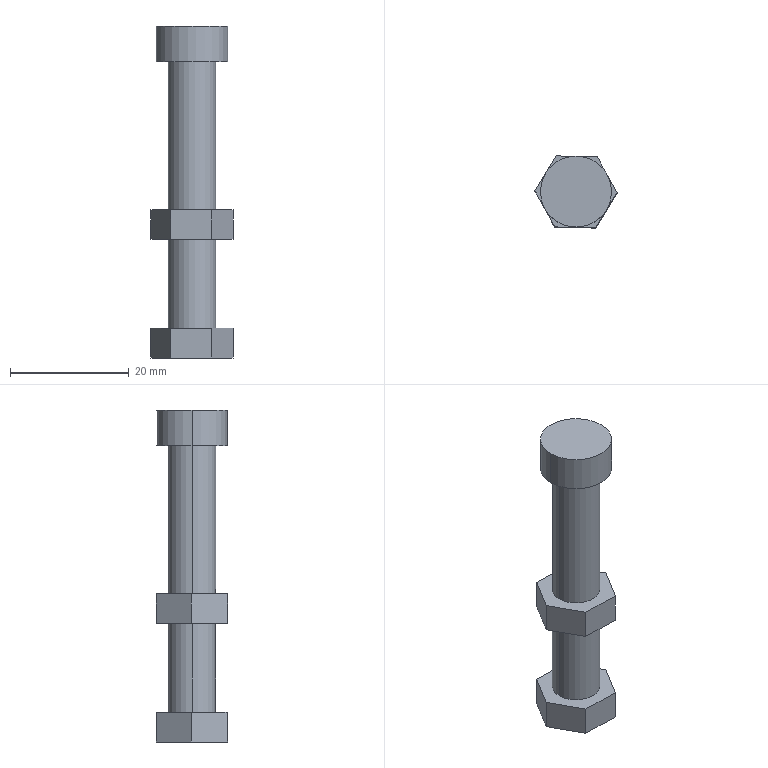Part | SolidWorks | features ICE 2, Extrusion 1, LPattern 1 | 1 solid | 24 faces | box 13.834 x 12.139 x 56 mm | volume 3933 mm3 | plane 18 | cylinder 6 | commonest cylinder face diameters 8 x4 12 x2
STEP:
#1=CARTESIAN_POINT('',(-4.,0.,20.));
#2=VERTEX_POINT('',#1);
#3=CARTESIAN_POINT('',(4.,0.,20.));
#4=VERTEX_POINT('',#3);
#5=CARTESIAN_POINT('',(0.,0.,20.));
#6=DIRECTION('',(0.,0.,-1.));
#7=DIRECTION('',(-1.,0.,0.));
#8=AXIS2_PLACEMENT_3D('',#5,#6,#7);
#9=CIRCLE('',#8,4.);
#10=EDGE_CURVE('',#2,#4,#9,.T.);
#11=ORIENTED_EDGE('',*,*,#10,.T.);
#12=CARTESIAN_POINT('',(4.,0.,5.));
#13=VERTEX_POINT('',#12);
#14=CARTESIAN_POINT('',(4.,0.,50.));
#15=DIRECTION('',(0.,0.,-1.));
#16=VECTOR('',#15,1000.);
#17=LINE('',#14,#16);
#18=EDGE_CURVE('',#4,#13,#17,.T.);
#19=ORIENTED_EDGE('',*,*,#18,.T.);
#20=CARTESIAN_POINT('',(-4.,0.,5.));
#21=VERTEX_POINT('',#20);
#22=CARTESIAN_POINT('',(0.,0.,5.));
#23=DIRECTION('',(0.,0.,-1.));
#24=DIRECTION('',(-1.,0.,0.));
#25=AXIS2_PLACEMENT_3D('',#22,#23,#24);
#26=CIRCLE('',#25,4.);
#27=EDGE_CURVE('',#21,#13,#26,.T.);
#28=ORIENTED_EDGE('',*,*,#27,.F.);
#29=CARTESIAN_POINT('',(-4.,0.,50.));
#30=DIRECTION('',(0.,0.,-1.));
#31=VECTOR('',#30,1000.);
#32=LINE('',#29,#31);
#33=EDGE_CURVE('',#2,#21,#32,.T.);
#34=ORIENTED_EDGE('',*,*,#33,.F.);
#35=EDGE_LOOP('',(#11,#19,#28,#34));
#36=FACE_OUTER_BOUND('',#35,.T.);
#37=CARTESIAN_POINT('',(0.,0.,50.));
#38=DIRECTION('',(0.,0.,-1.));
#39=DIRECTION('',(-1.,0.,0.));
#40=AXIS2_PLACEMENT_3D('',#37,#38,#39);
#41=CYLINDRICAL_SURFACE('',#40,4.);
#42=ADVANCED_FACE('',(#36),#41,.T.);
#43=CARTESIAN_POINT('',(6.,0.,56.));
#44=VERTEX_POINT('',#43);
#45=CARTESIAN_POINT('',(-6.,0.,56.));
#46=VERTEX_POINT('',#45);
#47=CARTESIAN_POINT('',(0.,0.,56.));
#48=DIRECTION('',(0.,0.,1.));
#49=DIRECTION('',(1.,0.,0.));
#50=AXIS2_PLACEMENT_3D('',#47,#48,#49);
#51=CIRCLE('',#50,6.);
#52=EDGE_CURVE('',#44,#46,#51,.T.);
#53=ORIENTED_EDGE('',*,*,#52,.F.);
#54=CARTESIAN_POINT('',(6.,0.,50.));
#55=VERTEX_POINT('',#54);
#56=CARTESIAN_POINT('',(6.,0.,56.));
#57=DIRECTION('',(0.,0.,-1.));
#58=VECTOR('',#57,1000.);
#59=LINE('',#56,#58);
#60=EDGE_CURVE('',#44,#55,#59,.T.);
#61=ORIENTED_EDGE('',*,*,#60,.T.);
#62=CARTESIAN_POINT('',(-6.,0.,50.));
#63=VERTEX_POINT('',#62);
#64=CARTESIAN_POINT('',(0.,0.,50.));
#65=DIRECTION('',(0.,0.,1.));
#66=DIRECTION('',(1.,0.,0.));
#67=AXIS2_PLACEMENT_3D('',#64,#65,#66);
#68=CIRCLE('',#67,6.);
#69=EDGE_CURVE('',#55,#63,#68,.T.);
#70=ORIENTED_EDGE('',*,*,#69,.T.);
#71=CARTESIAN_POINT('',(-6.,0.,56.));
#72=DIRECTION('',(0.,0.,-1.));
#73=VECTOR('',#72,1000.);
#74=LINE('',#71,#73);
#75=EDGE_CURVE('',#46,#63,#74,.T.);
#76=ORIENTED_EDGE('',*,*,#75,.F.);
#77=EDGE_LOOP('',(#53,#61,#70,#76));
#78=FACE_OUTER_BOUND('',#77,.T.);
#79=CARTESIAN_POINT('',(0.,0.,56.));
#80=DIRECTION('',(0.,0.,-1.));
#81=DIRECTION('',(-1.,0.,0.));
#82=AXIS2_PLACEMENT_3D('',#79,#80,#81);
#83=CYLINDRICAL_SURFACE('',#82,6.);
#84=ADVANCED_FACE('',(#78),#83,.T.);
#85=CARTESIAN_POINT('',(4.,0.,50.));
#86=VERTEX_POINT('',#85);
#87=CARTESIAN_POINT('',(-4.,0.,50.));
#88=VERTEX_POINT('',#87);
#89=CARTESIAN_POINT('',(0.,0.,50.));
#90=DIRECTION('',(0.,0.,1.));
#91=DIRECTION('',(1.,0.,0.));
#92=AXIS2_PLACEMENT_3D('',#89,#90,#91);
#93=CIRCLE('',#92,4.);
#94=EDGE_CURVE('',#86,#88,#93,.T.);
#95=ORIENTED_EDGE('',*,*,#94,.F.);
#96=CARTESIAN_POINT('',(4.,0.,25.));
#97=VERTEX_POINT('',#96);
#98=CARTESIAN_POINT('',(4.,0.,50.));
#99=DIRECTION('',(0.,0.,-1.));
#100=VECTOR('',#99,1000.);
#101=LINE('',#98,#100);
#102=EDGE_CURVE('',#86,#97,#101,.T.);
#103=ORIENTED_EDGE('',*,*,#102,.T.);
#104=CARTESIAN_POINT('',(-4.,0.,25.));
#105=VERTEX_POINT('',#104);
#106=CARTESIAN_POINT('',(0.,0.,25.));
#107=DIRECTION('',(0.,0.,-1.));
#108=DIRECTION('',(-1.,0.,0.));
#109=AXIS2_PLACEMENT_3D('',#106,#107,#108);
#110=CIRCLE('',#109,4.);
#111=EDGE_CURVE('',#105,#97,#110,.T.);
#112=ORIENTED_EDGE('',*,*,#111,.F.);
#113=CARTESIAN_POINT('',(-4.,0.,50.));
#114=DIRECTION('',(0.,0.,-1.));
#115=VECTOR('',#114,1000.);
#116=LINE('',#113,#115);
#117=EDGE_CURVE('',#88,#105,#116,.T.);
#118=ORIENTED_EDGE('',*,*,#117,.F.);
#119=EDGE_LOOP('',(#95,#103,#112,#118));
#120=FACE_OUTER_BOUND('',#119,.T.);
#121=CARTESIAN_POINT('',(0.,0.,50.));
#122=DIRECTION('',(0.,0.,-1.));
#123=DIRECTION('',(-1.,0.,0.));
#124=AXIS2_PLACEMENT_3D('',#121,#122,#123);
#125=CYLINDRICAL_SURFACE('',#124,4.);
#126=ADVANCED_FACE('',(#120),#125,.T.);
#127=ORIENTED_EDGE('',*,*,#102,.F.);
#128=CARTESIAN_POINT('',(0.,0.,50.));
#129=DIRECTION('',(0.,0.,1.));
#130=DIRECTION('',(1.,0.,0.));
#131=AXIS2_PLACEMENT_3D('',#128,#129,#130);
#132=CIRCLE('',#131,4.);
#133=EDGE_CURVE('',#88,#86,#132,.T.);
#134=ORIENTED_EDGE('',*,*,#133,.F.);
#135=ORIENTED_EDGE('',*,*,#117,.T.);
#136=CARTESIAN_POINT('',(0.,0.,25.));
#137=DIRECTION('',(0.,0.,-1.));
#138=DIRECTION('',(-1.,0.,0.));
#139=AXIS2_PLACEMENT_3D('',#136,#137,#138);
#140=CIRCLE('',#139,4.);
#141=EDGE_CURVE('',#97,#105,#140,.T.);
#142=ORIENTED_EDGE('',*,*,#141,.F.);
#143=EDGE_LOOP('',(#127,#134,#135,#142));
#144=FACE_OUTER_BOUND('',#143,.T.);
#145=CARTESIAN_POINT('',(0.,0.,50.));
#146=DIRECTION('',(0.,0.,-1.));
#147=DIRECTION('',(-1.,0.,0.));
#148=AXIS2_PLACEMENT_3D('',#145,#146,#147);
#149=CYLINDRICAL_SURFACE('',#148,4.);
#150=ADVANCED_FACE('',(#144),#149,.T.);
#151=ORIENTED_EDGE('',*,*,#60,.F.);
#152=CARTESIAN_POINT('',(0.,0.,56.));
#153=DIRECTION('',(0.,0.,1.));
#154=DIRECTION('',(1.,0.,0.));
#155=AXIS2_PLACEMENT_3D('',#152,#153,#154);
#156=CIRCLE('',#155,6.);
#157=EDGE_CURVE('',#46,#44,#156,.T.);
#158=ORIENTED_EDGE('',*,*,#157,.F.);
#159=ORIENTED_EDGE('',*,*,#75,.T.);
#160=CARTESIAN_POINT('',(0.,0.,50.));
#161=DIRECTION('',(0.,0.,1.));
#162=DIRECTION('',(1.,0.,0.));
#163=AXIS2_PLACEMENT_3D('',#160,#161,#162);
#164=CIRCLE('',#163,6.);
#165=EDGE_CURVE('',#63,#55,#164,.T.);
#166=ORIENTED_EDGE('',*,*,#165,.T.);
#167=EDGE_LOOP('',(#151,#158,#159,#166));
#168=FACE_OUTER_BOUND('',#167,.T.);
#169=CARTESIAN_POINT('',(0.,0.,56.));
#170=DIRECTION('',(0.,0.,-1.));
#171=DIRECTION('',(-1.,0.,0.));
#172=AXIS2_PLACEMENT_3D('',#169,#170,#171);
#173=CYLINDRICAL_SURFACE('',#172,6.);
#174=ADVANCED_FACE('',(#168),#173,.T.);
#175=ORIENTED_EDGE('',*,*,#157,.T.);
#176=ORIENTED_EDGE('',*,*,#52,.T.);
#177=EDGE_LOOP('',(#175,#176));
#178=FACE_OUTER_BOUND('',#177,.T.);
#179=CARTESIAN_POINT('',(0.,0.,56.));
#180=DIRECTION('',(0.,0.,1.));
#181=DIRECTION('',(1.,0.,0.));
#182=AXIS2_PLACEMENT_3D('',#179,#180,#181);
#183=PLANE('',#182);
#184=ADVANCED_FACE('',(#178),#183,.T.);
#185=ORIENTED_EDGE('',*,*,#133,.T.);
#186=ORIENTED_EDGE('',*,*,#94,.T.);
#187=EDGE_LOOP('',(#185,#186));
#188=FACE_BOUND('',#187,.T.);
#189=ORIENTED_EDGE('',*,*,#165,.F.);
#190=ORIENTED_EDGE('',*,*,#69,.F.);
#191=EDGE_LOOP('',(#189,#190));
#192=FACE_OUTER_BOUND('',#191,.T.);
#193=CARTESIAN_POINT('',(0.,0.,50.));
#194=DIRECTION('',(0.,0.,1.));
#195=DIRECTION('',(1.,0.,0.));
#196=AXIS2_PLACEMENT_3D('',#193,#194,#195);
#197=PLANE('',#196);
#198=ADVANCED_FACE('',(#188,#192),#197,.F.);
#199=CARTESIAN_POINT('',(-6.917,0.1581,20.));
#200=VERTEX_POINT('',#199);
#201=CARTESIAN_POINT('',(-3.322,6.069,20.));
#202=VERTEX_POINT('',#201);
#203=CARTESIAN_POINT('',(-6.917,0.1581,20.));
#204=DIRECTION('',(0.5197,0.8544,0.));
#205=VECTOR('',#204,1000.);
#206=LINE('',#203,#205);
#207=EDGE_CURVE('',#200,#202,#206,.T.);
#208=ORIENTED_EDGE('',*,*,#207,.F.);
#209=CARTESIAN_POINT('',(-6.917,0.1581,25.));
#210=VERTEX_POINT('',#209);
#211=CARTESIAN_POINT('',(-6.917,0.1581,25.));
#212=DIRECTION('',(0.,0.,-1.));
#213=VECTOR('',#212,1000.);
#214=LINE('',#211,#213);
#215=EDGE_CURVE('',#210,#200,#214,.T.);
#216=ORIENTED_EDGE('',*,*,#215,.F.);
#217=CARTESIAN_POINT('',(-3.322,6.069,25.));
#218=VERTEX_POINT('',#217);
#219=CARTESIAN_POINT('',(-6.917,0.1581,25.));
#220=DIRECTION('',(0.5197,0.8544,0.));
#221=VECTOR('',#220,1000.);
#222=LINE('',#219,#221);
#223=EDGE_CURVE('',#210,#218,#222,.T.);
#224=ORIENTED_EDGE('',*,*,#223,.T.);
#225=CARTESIAN_POINT('',(-3.322,6.069,25.));
#226=DIRECTION('',(0.,0.,-1.));
#227=VECTOR('',#226,1000.);
#228=LINE('',#225,#227);
#229=EDGE_CURVE('',#218,#202,#228,.T.);
#230=ORIENTED_EDGE('',*,*,#229,.T.);
#231=EDGE_LOOP('',(#208,#216,#224,#230));
#232=FACE_OUTER_BOUND('',#231,.T.);
#233=CARTESIAN_POINT('',(-6.917,0.1581,25.));
#234=DIRECTION('',(-0.8544,0.5197,0.));
#235=DIRECTION('',(-0.5197,-0.8544,0.));
#236=AXIS2_PLACEMENT_3D('',#233,#234,#235);
#237=PLANE('',#236);
#238=ADVANCED_FACE('',(#232),#237,.T.);
#239=CARTESIAN_POINT('',(-3.595,-5.911,20.));
#240=VERTEX_POINT('',#239);
#241=CARTESIAN_POINT('',(-3.595,-5.911,20.));
#242=DIRECTION('',(-0.4801,0.8772,0.));
#243=VECTOR('',#242,1000.);
#244=LINE('',#241,#243);
#245=EDGE_CURVE('',#240,#200,#244,.T.);
#246=ORIENTED_EDGE('',*,*,#245,.F.);
#247=CARTESIAN_POINT('',(-3.595,-5.911,25.));
#248=VERTEX_POINT('',#247);
#249=CARTESIAN_POINT('',(-3.595,-5.911,25.));
#250=DIRECTION('',(0.,0.,-1.));
#251=VECTOR('',#250,1000.);
#252=LINE('',#249,#251);
#253=EDGE_CURVE('',#248,#240,#252,.T.);
#254=ORIENTED_EDGE('',*,*,#253,.F.);
#255=CARTESIAN_POINT('',(-3.595,-5.911,25.));
#256=DIRECTION('',(-0.4801,0.8772,0.));
#257=VECTOR('',#256,1000.);
#258=LINE('',#255,#257);
#259=EDGE_CURVE('',#248,#210,#258,.T.);
#260=ORIENTED_EDGE('',*,*,#259,.T.);
#261=ORIENTED_EDGE('',*,*,#215,.T.);
#262=EDGE_LOOP('',(#246,#254,#260,#261));
#263=FACE_OUTER_BOUND('',#262,.T.);
#264=CARTESIAN_POINT('',(-3.595,-5.911,25.));
#265=DIRECTION('',(-0.8772,-0.4801,0.));
#266=DIRECTION('',(0.4801,-0.8772,0.));
#267=AXIS2_PLACEMENT_3D('',#264,#265,#266);
#268=PLANE('',#267);
#269=ADVANCED_FACE('',(#263),#268,.T.);
#270=CARTESIAN_POINT('',(3.322,-6.069,20.));
#271=VERTEX_POINT('',#270);
#272=CARTESIAN_POINT('',(3.322,-6.069,20.));
#273=DIRECTION('',(-0.9997,0.02285,0.));
#274=VECTOR('',#273,1000.);
#275=LINE('',#272,#274);
#276=EDGE_CURVE('',#271,#240,#275,.T.);
#277=ORIENTED_EDGE('',*,*,#276,.F.);
#278=CARTESIAN_POINT('',(3.322,-6.069,25.));
#279=VERTEX_POINT('',#278);
#280=CARTESIAN_POINT('',(3.322,-6.069,25.));
#281=DIRECTION('',(0.,0.,-1.));
#282=VECTOR('',#281,1000.);
#283=LINE('',#280,#282);
#284=EDGE_CURVE('',#279,#271,#283,.T.);
#285=ORIENTED_EDGE('',*,*,#284,.F.);
#286=CARTESIAN_POINT('',(3.322,-6.069,25.));
#287=DIRECTION('',(-0.9997,0.02285,0.));
#288=VECTOR('',#287,1000.);
#289=LINE('',#286,#288);
#290=EDGE_CURVE('',#279,#248,#289,.T.);
#291=ORIENTED_EDGE('',*,*,#290,.T.);
#292=ORIENTED_EDGE('',*,*,#253,.T.);
#293=EDGE_LOOP('',(#277,#285,#291,#292));
#294=FACE_OUTER_BOUND('',#293,.T.);
#295=CARTESIAN_POINT('',(3.322,-6.069,25.));
#296=DIRECTION('',(-0.02285,-0.9997,0.));
#297=DIRECTION('',(0.9997,-0.02285,0.));
#298=AXIS2_PLACEMENT_3D('',#295,#296,#297);
#299=PLANE('',#298);
#300=ADVANCED_FACE('',(#294),#299,.T.);
#301=CARTESIAN_POINT('',(6.917,-0.1581,20.));
#302=VERTEX_POINT('',#301);
#303=CARTESIAN_POINT('',(6.917,-0.1581,20.));
#304=DIRECTION('',(-0.5197,-0.8544,0.));
#305=VECTOR('',#304,1000.);
#306=LINE('',#303,#305);
#307=EDGE_CURVE('',#302,#271,#306,.T.);
#308=ORIENTED_EDGE('',*,*,#307,.F.);
#309=CARTESIAN_POINT('',(6.917,-0.1581,25.));
#310=VERTEX_POINT('',#309);
#311=CARTESIAN_POINT('',(6.917,-0.1581,25.));
#312=DIRECTION('',(0.,0.,-1.));
#313=VECTOR('',#312,1000.);
#314=LINE('',#311,#313);
#315=EDGE_CURVE('',#310,#302,#314,.T.);
#316=ORIENTED_EDGE('',*,*,#315,.F.);
#317=CARTESIAN_POINT('',(6.917,-0.1581,25.));
#318=DIRECTION('',(-0.5197,-0.8544,0.));
#319=VECTOR('',#318,1000.);
#320=LINE('',#317,#319);
#321=EDGE_CURVE('',#310,#279,#320,.T.);
#322=ORIENTED_EDGE('',*,*,#321,.T.);
#323=ORIENTED_EDGE('',*,*,#284,.T.);
#324=EDGE_LOOP('',(#308,#316,#322,#323));
#325=FACE_OUTER_BOUND('',#324,.T.);
#326=CARTESIAN_POINT('',(6.917,-0.1581,25.));
#327=DIRECTION('',(0.8544,-0.5197,0.));
#328=DIRECTION('',(0.5197,0.8544,0.));
#329=AXIS2_PLACEMENT_3D('',#326,#327,#328);
#330=PLANE('',#329);
#331=ADVANCED_FACE('',(#325),#330,.T.);
#332=CARTESIAN_POINT('',(3.595,5.911,20.));
#333=VERTEX_POINT('',#332);
#334=CARTESIAN_POINT('',(3.595,5.911,20.));
#335=DIRECTION('',(0.4801,-0.8772,0.));
#336=VECTOR('',#335,1000.);
#337=LINE('',#334,#336);
#338=EDGE_CURVE('',#333,#302,#337,.T.);
#339=ORIENTED_EDGE('',*,*,#338,.F.);
#340=CARTESIAN_POINT('',(3.595,5.911,25.));
#341=VERTEX_POINT('',#340);
#342=CARTESIAN_POINT('',(3.595,5.911,25.));
#343=DIRECTION('',(0.,0.,-1.));
#344=VECTOR('',#343,1000.);
#345=LINE('',#342,#344);
#346=EDGE_CURVE('',#341,#333,#345,.T.);
#347=ORIENTED_EDGE('',*,*,#346,.F.);
#348=CARTESIAN_POINT('',(3.595,5.911,25.));
#349=DIRECTION('',(0.4801,-0.8772,0.));
#350=VECTOR('',#349,1000.);
#351=LINE('',#348,#350);
#352=EDGE_CURVE('',#341,#310,#351,.T.);
#353=ORIENTED_EDGE('',*,*,#352,.T.);
#354=ORIENTED_EDGE('',*,*,#315,.T.);
#355=EDGE_LOOP('',(#339,#347,#353,#354));
#356=FACE_OUTER_BOUND('',#355,.T.);
#357=CARTESIAN_POINT('',(3.595,5.911,25.));
#358=DIRECTION('',(0.8772,0.4801,0.));
#359=DIRECTION('',(-0.4801,0.8772,0.));
#360=AXIS2_PLACEMENT_3D('',#357,#358,#359);
#361=PLANE('',#360);
#362=ADVANCED_FACE('',(#356),#361,.T.);
#363=CARTESIAN_POINT('',(-3.322,6.069,20.));
#364=DIRECTION('',(0.9997,-0.02285,0.));
#365=VECTOR('',#364,1000.);
#366=LINE('',#363,#365);
#367=EDGE_CURVE('',#202,#333,#366,.T.);
#368=ORIENTED_EDGE('',*,*,#367,.F.);
#369=ORIENTED_EDGE('',*,*,#229,.F.);
#370=CARTESIAN_POINT('',(-3.322,6.069,25.));
#371=DIRECTION('',(0.9997,-0.02285,0.));
#372=VECTOR('',#371,1000.);
#373=LINE('',#370,#372);
#374=EDGE_CURVE('',#218,#341,#373,.T.);
#375=ORIENTED_EDGE('',*,*,#374,.T.);
#376=ORIENTED_EDGE('',*,*,#346,.T.);
#377=EDGE_LOOP('',(#368,#369,#375,#376));
#378=FACE_OUTER_BOUND('',#377,.T.);
#379=CARTESIAN_POINT('',(-3.322,6.069,25.));
#380=DIRECTION('',(0.02285,0.9997,0.));
#381=DIRECTION('',(-0.9997,0.02285,0.));
#382=AXIS2_PLACEMENT_3D('',#379,#380,#381);
#383=PLANE('',#382);
#384=ADVANCED_FACE('',(#378),#383,.T.);
#385=ORIENTED_EDGE('',*,*,#111,.T.);
#386=ORIENTED_EDGE('',*,*,#141,.T.);
#387=EDGE_LOOP('',(#385,#386));
#388=FACE_BOUND('',#387,.T.);
#389=ORIENTED_EDGE('',*,*,#223,.F.);
#390=ORIENTED_EDGE('',*,*,#259,.F.);
#391=ORIENTED_EDGE('',*,*,#290,.F.);
#392=ORIENTED_EDGE('',*,*,#321,.F.);
#393=ORIENTED_EDGE('',*,*,#352,.F.);
#394=ORIENTED_EDGE('',*,*,#374,.F.);
#395=EDGE_LOOP('',(#389,#390,#391,#392,#393,#394));
#396=FACE_OUTER_BOUND('',#395,.T.);
#397=CARTESIAN_POINT('',(0.,0.,25.));
#398=DIRECTION('',(0.,0.,-1.));
#399=DIRECTION('',(-1.,0.,0.));
#400=AXIS2_PLACEMENT_3D('',#397,#398,#399);
#401=PLANE('',#400);
#402=ADVANCED_FACE('',(#388,#396),#401,.F.);
#403=ORIENTED_EDGE('',*,*,#10,.F.);
#404=CARTESIAN_POINT('',(0.,0.,20.));
#405=DIRECTION('',(0.,0.,-1.));
#406=DIRECTION('',(-1.,0.,0.));
#407=AXIS2_PLACEMENT_3D('',#404,#405,#406);
#408=CIRCLE('',#407,4.);
#409=EDGE_CURVE('',#4,#2,#408,.T.);
#410=ORIENTED_EDGE('',*,*,#409,.F.);
#411=EDGE_LOOP('',(#403,#410));
#412=FACE_BOUND('',#411,.T.);
#413=ORIENTED_EDGE('',*,*,#207,.T.);
#414=ORIENTED_EDGE('',*,*,#367,.T.);
#415=ORIENTED_EDGE('',*,*,#338,.T.);
#416=ORIENTED_EDGE('',*,*,#307,.T.);
#417=ORIENTED_EDGE('',*,*,#276,.T.);
#418=ORIENTED_EDGE('',*,*,#245,.T.);
#419=EDGE_LOOP('',(#413,#414,#415,#416,#417,#418));
#420=FACE_OUTER_BOUND('',#419,.T.);
#421=CARTESIAN_POINT('',(0.,0.,20.));
#422=DIRECTION('',(0.,0.,-1.));
#423=DIRECTION('',(-1.,0.,0.));
#424=AXIS2_PLACEMENT_3D('',#421,#422,#423);
#425=PLANE('',#424);
#426=ADVANCED_FACE('',(#412,#420),#425,.T.);
#427=CARTESIAN_POINT('',(-6.917,0.1581,0.));
#428=VERTEX_POINT('',#427);
#429=CARTESIAN_POINT('',(-3.322,6.069,0.));
#430=VERTEX_POINT('',#429);
#431=CARTESIAN_POINT('',(-6.917,0.1581,0.));
#432=DIRECTION('',(0.5197,0.8544,0.));
#433=VECTOR('',#432,1000.);
#434=LINE('',#431,#433);
#435=EDGE_CURVE('',#428,#430,#434,.T.);
#436=ORIENTED_EDGE('',*,*,#435,.T.);
#437=CARTESIAN_POINT('',(3.595,5.911,0.));
#438=VERTEX_POINT('',#437);
#439=CARTESIAN_POINT('',(-3.322,6.069,0.));
#440=DIRECTION('',(0.9997,-0.02285,0.));
#441=VECTOR('',#440,1000.);
#442=LINE('',#439,#441);
#443=EDGE_CURVE('',#430,#438,#442,.T.);
#444=ORIENTED_EDGE('',*,*,#443,.T.);
#445=CARTESIAN_POINT('',(6.917,-0.1581,0.));
#446=VERTEX_POINT('',#445);
#447=CARTESIAN_POINT('',(3.595,5.911,0.));
#448=DIRECTION('',(0.4801,-0.8772,0.));
#449=VECTOR('',#448,1000.);
#450=LINE('',#447,#449);
#451=EDGE_CURVE('',#438,#446,#450,.T.);
#452=ORIENTED_EDGE('',*,*,#451,.T.);
#453=CARTESIAN_POINT('',(3.322,-6.069,0.));
#454=VERTEX_POINT('',#453);
#455=CARTESIAN_POINT('',(6.917,-0.1581,0.));
#456=DIRECTION('',(-0.5197,-0.8544,0.));
#457=VECTOR('',#456,1000.);
#458=LINE('',#455,#457);
#459=EDGE_CURVE('',#446,#454,#458,.T.);
#460=ORIENTED_EDGE('',*,*,#459,.T.);
#461=CARTESIAN_POINT('',(-3.595,-5.911,0.));
#462=VERTEX_POINT('',#461);
#463=CARTESIAN_POINT('',(3.322,-6.069,0.));
#464=DIRECTION('',(-0.9997,0.02285,0.));
#465=VECTOR('',#464,1000.);
#466=LINE('',#463,#465);
#467=EDGE_CURVE('',#454,#462,#466,.T.);
#468=ORIENTED_EDGE('',*,*,#467,.T.);
#469=CARTESIAN_POINT('',(-3.595,-5.911,0.));
#470=DIRECTION('',(-0.4801,0.8772,0.));
#471=VECTOR('',#470,1000.);
#472=LINE('',#469,#471);
#473=EDGE_CURVE('',#462,#428,#472,.T.);
#474=ORIENTED_EDGE('',*,*,#473,.T.);
#475=EDGE_LOOP('',(#436,#444,#452,#460,#468,#474));
#476=FACE_OUTER_BOUND('',#475,.T.);
#477=CARTESIAN_POINT('',(0.,0.,0.));
#478=DIRECTION('',(0.,0.,1.));
#479=DIRECTION('',(1.,0.,0.));
#480=AXIS2_PLACEMENT_3D('',#477,#478,#479);
#481=PLANE('',#480);
#482=ADVANCED_FACE('',(#476),#481,.F.);
#483=ORIENTED_EDGE('',*,*,#443,.F.);
#484=CARTESIAN_POINT('',(-3.322,6.069,5.));
#485=VERTEX_POINT('',#484);
#486=CARTESIAN_POINT('',(-3.322,6.069,5.));
#487=DIRECTION('',(0.,0.,-1.));
#488=VECTOR('',#487,1000.);
#489=LINE('',#486,#488);
#490=EDGE_CURVE('',#485,#430,#489,.T.);
#491=ORIENTED_EDGE('',*,*,#490,.F.);
#492=CARTESIAN_POINT('',(3.595,5.911,5.));
#493=VERTEX_POINT('',#492);
#494=CARTESIAN_POINT('',(-3.322,6.069,5.));
#495=DIRECTION('',(0.9997,-0.02285,0.));
#496=VECTOR('',#495,1000.);
#497=LINE('',#494,#496);
#498=EDGE_CURVE('',#485,#493,#497,.T.);
#499=ORIENTED_EDGE('',*,*,#498,.T.);
#500=CARTESIAN_POINT('',(3.595,5.911,5.));
#501=DIRECTION('',(0.,0.,-1.));
#502=VECTOR('',#501,1000.);
#503=LINE('',#500,#502);
#504=EDGE_CURVE('',#493,#438,#503,.T.);
#505=ORIENTED_EDGE('',*,*,#504,.T.);
#506=EDGE_LOOP('',(#483,#491,#499,#505));
#507=FACE_OUTER_BOUND('',#506,.T.);
#508=CARTESIAN_POINT('',(-3.322,6.069,5.));
#509=DIRECTION('',(0.02285,0.9997,0.));
#510=DIRECTION('',(-0.9997,0.02285,0.));
#511=AXIS2_PLACEMENT_3D('',#508,#509,#510);
#512=PLANE('',#511);
#513=ADVANCED_FACE('',(#507),#512,.T.);
#514=ORIENTED_EDGE('',*,*,#451,.F.);
#515=ORIENTED_EDGE('',*,*,#504,.F.);
#516=CARTESIAN_POINT('',(6.917,-0.1581,5.));
#517=VERTEX_POINT('',#516);
#518=CARTESIAN_POINT('',(3.595,5.911,5.));
#519=DIRECTION('',(0.4801,-0.8772,0.));
#520=VECTOR('',#519,1000.);
#521=LINE('',#518,#520);
#522=EDGE_CURVE('',#493,#517,#521,.T.);
#523=ORIENTED_EDGE('',*,*,#522,.T.);
#524=CARTESIAN_POINT('',(6.917,-0.1581,5.));
#525=DIRECTION('',(0.,0.,-1.));
#526=VECTOR('',#525,1000.);
#527=LINE('',#524,#526);
#528=EDGE_CURVE('',#517,#446,#527,.T.);
#529=ORIENTED_EDGE('',*,*,#528,.T.);
#530=EDGE_LOOP('',(#514,#515,#523,#529));
#531=FACE_OUTER_BOUND('',#530,.T.);
#532=CARTESIAN_POINT('',(3.595,5.911,5.));
#533=DIRECTION('',(0.8772,0.4801,0.));
#534=DIRECTION('',(-0.4801,0.8772,0.));
#535=AXIS2_PLACEMENT_3D('',#532,#533,#534);
#536=PLANE('',#535);
#537=ADVANCED_FACE('',(#531),#536,.T.);
#538=ORIENTED_EDGE('',*,*,#459,.F.);
#539=ORIENTED_EDGE('',*,*,#528,.F.);
#540=CARTESIAN_POINT('',(3.322,-6.069,5.));
#541=VERTEX_POINT('',#540);
#542=CARTESIAN_POINT('',(6.917,-0.1581,5.));
#543=DIRECTION('',(-0.5197,-0.8544,0.));
#544=VECTOR('',#543,1000.);
#545=LINE('',#542,#544);
#546=EDGE_CURVE('',#517,#541,#545,.T.);
#547=ORIENTED_EDGE('',*,*,#546,.T.);
#548=CARTESIAN_POINT('',(3.322,-6.069,5.));
#549=DIRECTION('',(0.,0.,-1.));
#550=VECTOR('',#549,1000.);
#551=LINE('',#548,#550);
#552=EDGE_CURVE('',#541,#454,#551,.T.);
#553=ORIENTED_EDGE('',*,*,#552,.T.);
#554=EDGE_LOOP('',(#538,#539,#547,#553));
#555=FACE_OUTER_BOUND('',#554,.T.);
#556=CARTESIAN_POINT('',(6.917,-0.1581,5.));
#557=DIRECTION('',(0.8544,-0.5197,0.));
#558=DIRECTION('',(0.5197,0.8544,0.));
#559=AXIS2_PLACEMENT_3D('',#556,#557,#558);
#560=PLANE('',#559);
#561=ADVANCED_FACE('',(#555),#560,.T.);
#562=ORIENTED_EDGE('',*,*,#467,.F.);
#563=ORIENTED_EDGE('',*,*,#552,.F.);
#564=CARTESIAN_POINT('',(-3.595,-5.911,5.));
#565=VERTEX_POINT('',#564);
#566=CARTESIAN_POINT('',(3.322,-6.069,5.));
#567=DIRECTION('',(-0.9997,0.02285,0.));
#568=VECTOR('',#567,1000.);
#569=LINE('',#566,#568);
#570=EDGE_CURVE('',#541,#565,#569,.T.);
#571=ORIENTED_EDGE('',*,*,#570,.T.);
#572=CARTESIAN_POINT('',(-3.595,-5.911,5.));
#573=DIRECTION('',(0.,0.,-1.));
#574=VECTOR('',#573,1000.);
#575=LINE('',#572,#574);
#576=EDGE_CURVE('',#565,#462,#575,.T.);
#577=ORIENTED_EDGE('',*,*,#576,.T.);
#578=EDGE_LOOP('',(#562,#563,#571,#577));
#579=FACE_OUTER_BOUND('',#578,.T.);
#580=CARTESIAN_POINT('',(3.322,-6.069,5.));
#581=DIRECTION('',(-0.02285,-0.9997,0.));
#582=DIRECTION('',(0.9997,-0.02285,0.));
#583=AXIS2_PLACEMENT_3D('',#580,#581,#582);
#584=PLANE('',#583);
#585=ADVANCED_FACE('',(#579),#584,.T.);
#586=ORIENTED_EDGE('',*,*,#473,.F.);
#587=ORIENTED_EDGE('',*,*,#576,.F.);
#588=CARTESIAN_POINT('',(-6.917,0.1581,5.));
#589=VERTEX_POINT('',#588);
#590=CARTESIAN_POINT('',(-3.595,-5.911,5.));
#591=DIRECTION('',(-0.4801,0.8772,0.));
#592=VECTOR('',#591,1000.);
#593=LINE('',#590,#592);
#594=EDGE_CURVE('',#565,#589,#593,.T.);
#595=ORIENTED_EDGE('',*,*,#594,.T.);
#596=CARTESIAN_POINT('',(-6.917,0.1581,5.));
#597=DIRECTION('',(0.,0.,-1.));
#598=VECTOR('',#597,1000.);
#599=LINE('',#596,#598);
#600=EDGE_CURVE('',#589,#428,#599,.T.);
#601=ORIENTED_EDGE('',*,*,#600,.T.);
#602=EDGE_LOOP('',(#586,#587,#595,#601));
#603=FACE_OUTER_BOUND('',#602,.T.);
#604=CARTESIAN_POINT('',(-3.595,-5.911,5.));
#605=DIRECTION('',(-0.8772,-0.4801,0.));
#606=DIRECTION('',(0.4801,-0.8772,0.));
#607=AXIS2_PLACEMENT_3D('',#604,#605,#606);
#608=PLANE('',#607);
#609=ADVANCED_FACE('',(#603),#608,.T.);
#610=ORIENTED_EDGE('',*,*,#435,.F.);
#611=ORIENTED_EDGE('',*,*,#600,.F.);
#612=CARTESIAN_POINT('',(-6.917,0.1581,5.));
#613=DIRECTION('',(0.5197,0.8544,0.));
#614=VECTOR('',#613,1000.);
#615=LINE('',#612,#614);
#616=EDGE_CURVE('',#589,#485,#615,.T.);
#617=ORIENTED_EDGE('',*,*,#616,.T.);
#618=ORIENTED_EDGE('',*,*,#490,.T.);
#619=EDGE_LOOP('',(#610,#611,#617,#618));
#620=FACE_OUTER_BOUND('',#619,.T.);
#621=CARTESIAN_POINT('',(-6.917,0.1581,5.));
#622=DIRECTION('',(-0.8544,0.5197,0.));
#623=DIRECTION('',(-0.5197,-0.8544,0.));
#624=AXIS2_PLACEMENT_3D('',#621,#622,#623);
#625=PLANE('',#624);
#626=ADVANCED_FACE('',(#620),#625,.T.);
#627=ORIENTED_EDGE('',*,*,#27,.T.);
#628=CARTESIAN_POINT('',(0.,0.,5.));
#629=DIRECTION('',(0.,0.,-1.));
#630=DIRECTION('',(-1.,0.,0.));
#631=AXIS2_PLACEMENT_3D('',#628,#629,#630);
#632=CIRCLE('',#631,4.);
#633=EDGE_CURVE('',#13,#21,#632,.T.);
#634=ORIENTED_EDGE('',*,*,#633,.T.);
#635=EDGE_LOOP('',(#627,#634));
#636=FACE_BOUND('',#635,.T.);
#637=ORIENTED_EDGE('',*,*,#616,.F.);
#638=ORIENTED_EDGE('',*,*,#594,.F.);
#639=ORIENTED_EDGE('',*,*,#570,.F.);
#640=ORIENTED_EDGE('',*,*,#546,.F.);
#641=ORIENTED_EDGE('',*,*,#522,.F.);
#642=ORIENTED_EDGE('',*,*,#498,.F.);
#643=EDGE_LOOP('',(#637,#638,#639,#640,#641,#642));
#644=FACE_OUTER_BOUND('',#643,.T.);
#645=CARTESIAN_POINT('',(0.,0.,5.));
#646=DIRECTION('',(0.,0.,-1.));
#647=DIRECTION('',(-1.,0.,0.));
#648=AXIS2_PLACEMENT_3D('',#645,#646,#647);
#649=PLANE('',#648);
#650=ADVANCED_FACE('',(#636,#644),#649,.F.);
#651=ORIENTED_EDGE('',*,*,#18,.F.);
#652=ORIENTED_EDGE('',*,*,#409,.T.);
#653=ORIENTED_EDGE('',*,*,#33,.T.);
#654=ORIENTED_EDGE('',*,*,#633,.F.);
#655=EDGE_LOOP('',(#651,#652,#653,#654));
#656=FACE_OUTER_BOUND('',#655,.T.);
#657=CARTESIAN_POINT('',(0.,0.,50.));
#658=DIRECTION('',(0.,0.,-1.));
#659=DIRECTION('',(-1.,0.,0.));
#660=AXIS2_PLACEMENT_3D('',#657,#658,#659);
#661=CYLINDRICAL_SURFACE('',#660,4.);
#662=ADVANCED_FACE('',(#656),#661,.T.);
#663=CLOSED_SHELL('',(#42,#84,#126,#150,#174,#184,#198,#238,#269,#300,#331,#362,#384,#402,#426,#482,#513,#537,#561,#585,#609,#626,#650,#662));
#664=MANIFOLD_SOLID_BREP('',#663);
#665=CARTESIAN_POINT('',(0.,0.,0.));
#666=DIRECTION('',(0.,0.,1.));
#667=DIRECTION('',(1.,0.,0.));
#668=AXIS2_PLACEMENT_3D('',#665,#666,#667);
#669=(LENGTH_UNIT()NAMED_UNIT(*)SI_UNIT(.MILLI.,.METRE.));
#670=UNCERTAINTY_MEASURE_WITH_UNIT(LENGTH_MEASURE(0.00001),#669,'','');
#671=(NAMED_UNIT(*)PLANE_ANGLE_UNIT()SI_UNIT($,.RADIAN.));
#672=(NAMED_UNIT(*)SI_UNIT($,.STERADIAN.)SOLID_ANGLE_UNIT());
#673=(GEOMETRIC_REPRESENTATION_CONTEXT(3)GLOBAL_UNCERTAINTY_ASSIGNED_CONTEXT((#670))GLOBAL_UNIT_ASSIGNED_CONTEXT((#669,#671,#672))REPRESENTATION_CONTEXT('',''));
#674=ADVANCED_BREP_SHAPE_REPRESENTATION('',(#664,#668),#673);